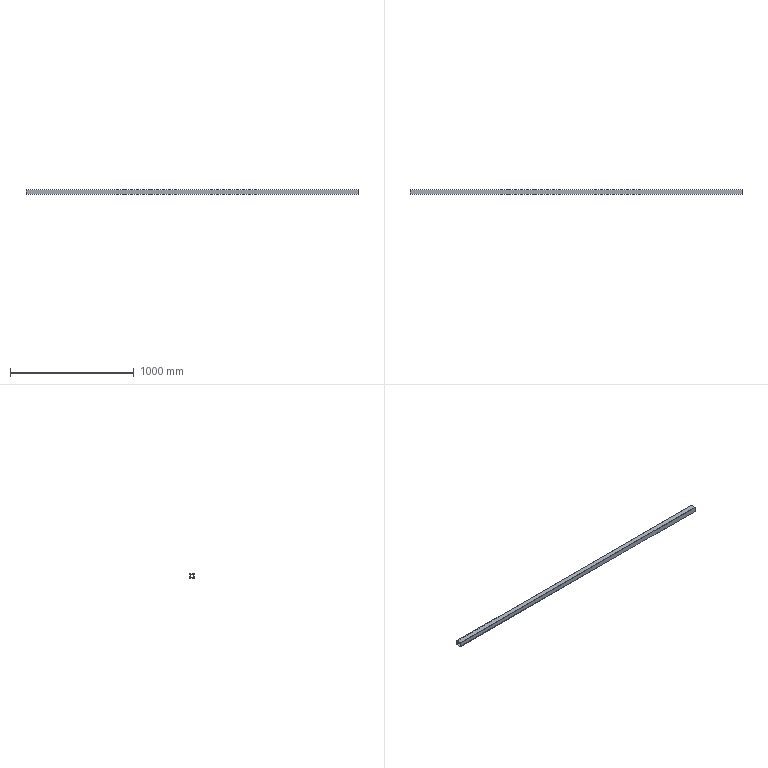Part | NX | features solid 2 | 1 solid | 10 faces | box 2680 x 40 x 40 mm | volume 1543680 mm3 | plane 10
STEP:
#1=CARTESIAN_POINT('',(1140.,-370.,-45.));
#2=VERTEX_POINT('',#1);
#3=CARTESIAN_POINT('',(1140.,-370.,-85.));
#4=VERTEX_POINT('',#3);
#5=CARTESIAN_POINT('',(1140.,-370.,-70.));
#6=DIRECTION('',(0.,0.,-1.));
#7=VECTOR('',#6,1000.);
#8=LINE('',#5,#7);
#9=EDGE_CURVE('',#2,#4,#8,.T.);
#10=ORIENTED_EDGE('',*,*,#9,.F.);
#11=CARTESIAN_POINT('',(-1540.,-370.,-45.));
#12=VERTEX_POINT('',#11);
#13=CARTESIAN_POINT('',(204.393,-370.,-45.));
#14=DIRECTION('',(1.,0.,0.));
#15=VECTOR('',#14,1000.);
#16=LINE('',#13,#15);
#17=EDGE_CURVE('',#12,#2,#16,.T.);
#18=ORIENTED_EDGE('',*,*,#17,.F.);
#19=CARTESIAN_POINT('',(-1540.,-370.,-85.));
#20=VERTEX_POINT('',#19);
#21=CARTESIAN_POINT('',(-1540.,-370.,-70.));
#22=DIRECTION('',(0.,0.,-1.));
#23=VECTOR('',#22,1000.);
#24=LINE('',#21,#23);
#25=EDGE_CURVE('',#12,#20,#24,.T.);
#26=ORIENTED_EDGE('',*,*,#25,.T.);
#27=CARTESIAN_POINT('',(119.393,-370.,-85.));
#28=DIRECTION('',(1.,0.,0.));
#29=VECTOR('',#28,1000.);
#30=LINE('',#27,#29);
#31=EDGE_CURVE('',#20,#4,#30,.T.);
#32=ORIENTED_EDGE('',*,*,#31,.T.);
#33=EDGE_LOOP('',(#10,#18,#26,#32));
#34=FACE_BOUND('',#33,.T.);
#35=CARTESIAN_POINT('',(119.393,-370.,-70.));
#36=DIRECTION('',(0.,1.,0.));
#37=DIRECTION('',(0.,0.,1.));
#38=AXIS2_PLACEMENT_3D('',#35,#36,#37);
#39=PLANE('',#38);
#40=ADVANCED_FACE('',(#34),#39,.F.);
#41=CARTESIAN_POINT('',(1140.,-330.,-85.));
#42=VERTEX_POINT('',#41);
#43=CARTESIAN_POINT('',(1140.,-950.,-85.));
#44=DIRECTION('',(0.,1.,0.));
#45=VECTOR('',#44,1000.);
#46=LINE('',#43,#45);
#47=EDGE_CURVE('',#4,#42,#46,.T.);
#48=ORIENTED_EDGE('',*,*,#47,.F.);
#49=ORIENTED_EDGE('',*,*,#31,.F.);
#50=CARTESIAN_POINT('',(-1540.,-330.,-85.));
#51=VERTEX_POINT('',#50);
#52=CARTESIAN_POINT('',(-1540.,-950.,-85.));
#53=DIRECTION('',(0.,1.,0.));
#54=VECTOR('',#53,1000.);
#55=LINE('',#52,#54);
#56=EDGE_CURVE('',#20,#51,#55,.T.);
#57=ORIENTED_EDGE('',*,*,#56,.T.);
#58=CARTESIAN_POINT('',(204.393,-330.,-85.));
#59=DIRECTION('',(1.,0.,0.));
#60=VECTOR('',#59,1000.);
#61=LINE('',#58,#60);
#62=EDGE_CURVE('',#51,#42,#61,.T.);
#63=ORIENTED_EDGE('',*,*,#62,.T.);
#64=EDGE_LOOP('',(#48,#49,#57,#63));
#65=FACE_BOUND('',#64,.T.);
#66=CARTESIAN_POINT('',(204.393,-950.,-85.));
#67=DIRECTION('',(0.,0.,1.));
#68=DIRECTION('',(0.,-1.,0.));
#69=AXIS2_PLACEMENT_3D('',#66,#67,#68);
#70=PLANE('',#69);
#71=ADVANCED_FACE('',(#65),#70,.F.);
#72=CARTESIAN_POINT('',(1140.,-330.,-45.));
#73=VERTEX_POINT('',#72);
#74=CARTESIAN_POINT('',(1140.,-990.,-45.));
#75=DIRECTION('',(0.,-1.,0.));
#76=VECTOR('',#75,1000.);
#77=LINE('',#74,#76);
#78=EDGE_CURVE('',#73,#2,#77,.T.);
#79=ORIENTED_EDGE('',*,*,#78,.F.);
#80=CARTESIAN_POINT('',(-1540.,-330.,-45.));
#81=VERTEX_POINT('',#80);
#82=CARTESIAN_POINT('',(204.393,-330.,-45.));
#83=DIRECTION('',(-1.,0.,0.));
#84=VECTOR('',#83,1000.);
#85=LINE('',#82,#84);
#86=EDGE_CURVE('',#73,#81,#85,.T.);
#87=ORIENTED_EDGE('',*,*,#86,.T.);
#88=CARTESIAN_POINT('',(-1540.,-990.,-45.));
#89=DIRECTION('',(0.,-1.,0.));
#90=VECTOR('',#89,1000.);
#91=LINE('',#88,#90);
#92=EDGE_CURVE('',#81,#12,#91,.T.);
#93=ORIENTED_EDGE('',*,*,#92,.T.);
#94=ORIENTED_EDGE('',*,*,#17,.T.);
#95=EDGE_LOOP('',(#79,#87,#93,#94));
#96=FACE_BOUND('',#95,.T.);
#97=CARTESIAN_POINT('',(204.393,-990.,-45.));
#98=DIRECTION('',(0.,0.,-1.));
#99=DIRECTION('',(0.,1.,0.));
#100=AXIS2_PLACEMENT_3D('',#97,#98,#99);
#101=PLANE('',#100);
#102=ADVANCED_FACE('',(#96),#101,.F.);
#103=CARTESIAN_POINT('',(1140.,-330.,-40.));
#104=DIRECTION('',(0.,0.,1.));
#105=VECTOR('',#104,1000.);
#106=LINE('',#103,#105);
#107=EDGE_CURVE('',#42,#73,#106,.T.);
#108=ORIENTED_EDGE('',*,*,#107,.F.);
#109=ORIENTED_EDGE('',*,*,#62,.F.);
#110=CARTESIAN_POINT('',(-1540.,-330.,-40.));
#111=DIRECTION('',(0.,0.,1.));
#112=VECTOR('',#111,1000.);
#113=LINE('',#110,#112);
#114=EDGE_CURVE('',#51,#81,#113,.T.);
#115=ORIENTED_EDGE('',*,*,#114,.T.);
#116=ORIENTED_EDGE('',*,*,#86,.F.);
#117=EDGE_LOOP('',(#108,#109,#115,#116));
#118=FACE_BOUND('',#117,.T.);
#119=CARTESIAN_POINT('',(119.393,-330.,-40.));
#120=DIRECTION('',(0.,-1.,0.));
#121=DIRECTION('',(0.,0.,-1.));
#122=AXIS2_PLACEMENT_3D('',#119,#120,#121);
#123=PLANE('',#122);
#124=ADVANCED_FACE('',(#118),#123,.F.);
#125=CARTESIAN_POINT('',(-1540.,-366.,-49.));
#126=VERTEX_POINT('',#125);
#127=CARTESIAN_POINT('',(1140.,-366.,-49.));
#128=VERTEX_POINT('',#127);
#129=CARTESIAN_POINT('',(204.393,-366.,-49.));
#130=DIRECTION('',(1.,0.,0.));
#131=VECTOR('',#130,1000.);
#132=LINE('',#129,#131);
#133=EDGE_CURVE('',#126,#128,#132,.T.);
#134=ORIENTED_EDGE('',*,*,#133,.T.);
#135=CARTESIAN_POINT('',(1140.,-366.,-81.));
#136=VERTEX_POINT('',#135);
#137=CARTESIAN_POINT('',(1140.,-366.,-70.));
#138=DIRECTION('',(0.,0.,-1.));
#139=VECTOR('',#138,1000.);
#140=LINE('',#137,#139);
#141=EDGE_CURVE('',#128,#136,#140,.T.);
#142=ORIENTED_EDGE('',*,*,#141,.T.);
#143=CARTESIAN_POINT('',(-1540.,-366.,-81.));
#144=VERTEX_POINT('',#143);
#145=CARTESIAN_POINT('',(119.393,-366.,-81.));
#146=DIRECTION('',(1.,0.,0.));
#147=VECTOR('',#146,1000.);
#148=LINE('',#145,#147);
#149=EDGE_CURVE('',#144,#136,#148,.T.);
#150=ORIENTED_EDGE('',*,*,#149,.F.);
#151=CARTESIAN_POINT('',(-1540.,-366.,-70.));
#152=DIRECTION('',(0.,0.,-1.));
#153=VECTOR('',#152,1000.);
#154=LINE('',#151,#153);
#155=EDGE_CURVE('',#126,#144,#154,.T.);
#156=ORIENTED_EDGE('',*,*,#155,.F.);
#157=EDGE_LOOP('',(#134,#142,#150,#156));
#158=FACE_BOUND('',#157,.T.);
#159=CARTESIAN_POINT('',(119.393,-366.,-70.));
#160=DIRECTION('',(0.,1.,0.));
#161=DIRECTION('',(0.,0.,1.));
#162=AXIS2_PLACEMENT_3D('',#159,#160,#161);
#163=PLANE('',#162);
#164=ADVANCED_FACE('',(#158),#163,.T.);
#165=ORIENTED_EDGE('',*,*,#149,.T.);
#166=CARTESIAN_POINT('',(1140.,-334.,-81.));
#167=VERTEX_POINT('',#166);
#168=CARTESIAN_POINT('',(1140.,-950.,-81.));
#169=DIRECTION('',(0.,1.,0.));
#170=VECTOR('',#169,1000.);
#171=LINE('',#168,#170);
#172=EDGE_CURVE('',#136,#167,#171,.T.);
#173=ORIENTED_EDGE('',*,*,#172,.T.);
#174=CARTESIAN_POINT('',(-1540.,-334.,-81.));
#175=VERTEX_POINT('',#174);
#176=CARTESIAN_POINT('',(204.393,-334.,-81.));
#177=DIRECTION('',(1.,0.,0.));
#178=VECTOR('',#177,1000.);
#179=LINE('',#176,#178);
#180=EDGE_CURVE('',#175,#167,#179,.T.);
#181=ORIENTED_EDGE('',*,*,#180,.F.);
#182=CARTESIAN_POINT('',(-1540.,-950.,-81.));
#183=DIRECTION('',(0.,1.,0.));
#184=VECTOR('',#183,1000.);
#185=LINE('',#182,#184);
#186=EDGE_CURVE('',#144,#175,#185,.T.);
#187=ORIENTED_EDGE('',*,*,#186,.F.);
#188=EDGE_LOOP('',(#165,#173,#181,#187));
#189=FACE_BOUND('',#188,.T.);
#190=CARTESIAN_POINT('',(204.393,-950.,-81.));
#191=DIRECTION('',(0.,0.,1.));
#192=DIRECTION('',(0.,-1.,0.));
#193=AXIS2_PLACEMENT_3D('',#190,#191,#192);
#194=PLANE('',#193);
#195=ADVANCED_FACE('',(#189),#194,.T.);
#196=CARTESIAN_POINT('',(1140.,-334.,-49.));
#197=VERTEX_POINT('',#196);
#198=CARTESIAN_POINT('',(-1540.,-334.,-49.));
#199=VERTEX_POINT('',#198);
#200=CARTESIAN_POINT('',(204.393,-334.,-49.));
#201=DIRECTION('',(-1.,0.,0.));
#202=VECTOR('',#201,1000.);
#203=LINE('',#200,#202);
#204=EDGE_CURVE('',#197,#199,#203,.T.);
#205=ORIENTED_EDGE('',*,*,#204,.F.);
#206=CARTESIAN_POINT('',(1140.,-990.,-49.));
#207=DIRECTION('',(0.,-1.,0.));
#208=VECTOR('',#207,1000.);
#209=LINE('',#206,#208);
#210=EDGE_CURVE('',#197,#128,#209,.T.);
#211=ORIENTED_EDGE('',*,*,#210,.T.);
#212=ORIENTED_EDGE('',*,*,#133,.F.);
#213=CARTESIAN_POINT('',(-1540.,-990.,-49.));
#214=DIRECTION('',(0.,-1.,0.));
#215=VECTOR('',#214,1000.);
#216=LINE('',#213,#215);
#217=EDGE_CURVE('',#199,#126,#216,.T.);
#218=ORIENTED_EDGE('',*,*,#217,.F.);
#219=EDGE_LOOP('',(#205,#211,#212,#218));
#220=FACE_BOUND('',#219,.T.);
#221=CARTESIAN_POINT('',(204.393,-990.,-49.));
#222=DIRECTION('',(0.,0.,-1.));
#223=DIRECTION('',(0.,1.,0.));
#224=AXIS2_PLACEMENT_3D('',#221,#222,#223);
#225=PLANE('',#224);
#226=ADVANCED_FACE('',(#220),#225,.T.);
#227=ORIENTED_EDGE('',*,*,#180,.T.);
#228=CARTESIAN_POINT('',(1140.,-334.,-40.));
#229=DIRECTION('',(0.,0.,1.));
#230=VECTOR('',#229,1000.);
#231=LINE('',#228,#230);
#232=EDGE_CURVE('',#167,#197,#231,.T.);
#233=ORIENTED_EDGE('',*,*,#232,.T.);
#234=ORIENTED_EDGE('',*,*,#204,.T.);
#235=CARTESIAN_POINT('',(-1540.,-334.,-40.));
#236=DIRECTION('',(0.,0.,1.));
#237=VECTOR('',#236,1000.);
#238=LINE('',#235,#237);
#239=EDGE_CURVE('',#175,#199,#238,.T.);
#240=ORIENTED_EDGE('',*,*,#239,.F.);
#241=EDGE_LOOP('',(#227,#233,#234,#240));
#242=FACE_BOUND('',#241,.T.);
#243=CARTESIAN_POINT('',(119.393,-334.,-40.));
#244=DIRECTION('',(0.,-1.,0.));
#245=DIRECTION('',(0.,0.,-1.));
#246=AXIS2_PLACEMENT_3D('',#243,#244,#245);
#247=PLANE('',#246);
#248=ADVANCED_FACE('',(#242),#247,.T.);
#249=ORIENTED_EDGE('',*,*,#217,.T.);
#250=ORIENTED_EDGE('',*,*,#155,.T.);
#251=ORIENTED_EDGE('',*,*,#186,.T.);
#252=ORIENTED_EDGE('',*,*,#239,.T.);
#253=EDGE_LOOP('',(#249,#250,#251,#252));
#254=FACE_BOUND('',#253,.T.);
#255=ORIENTED_EDGE('',*,*,#25,.F.);
#256=ORIENTED_EDGE('',*,*,#92,.F.);
#257=ORIENTED_EDGE('',*,*,#114,.F.);
#258=ORIENTED_EDGE('',*,*,#56,.F.);
#259=EDGE_LOOP('',(#255,#256,#257,#258));
#260=FACE_BOUND('',#259,.T.);
#261=CARTESIAN_POINT('',(-1540.,180.,-39.5));
#262=DIRECTION('',(1.,0.,0.));
#263=DIRECTION('',(0.,-1.,0.));
#264=AXIS2_PLACEMENT_3D('',#261,#262,#263);
#265=PLANE('',#264);
#266=ADVANCED_FACE('',(#254,#260),#265,.F.);
#267=ORIENTED_EDGE('',*,*,#141,.F.);
#268=ORIENTED_EDGE('',*,*,#210,.F.);
#269=ORIENTED_EDGE('',*,*,#232,.F.);
#270=ORIENTED_EDGE('',*,*,#172,.F.);
#271=EDGE_LOOP('',(#267,#268,#269,#270));
#272=FACE_BOUND('',#271,.T.);
#273=ORIENTED_EDGE('',*,*,#78,.T.);
#274=ORIENTED_EDGE('',*,*,#9,.T.);
#275=ORIENTED_EDGE('',*,*,#47,.T.);
#276=ORIENTED_EDGE('',*,*,#107,.T.);
#277=EDGE_LOOP('',(#273,#274,#275,#276));
#278=FACE_BOUND('',#277,.T.);
#279=CARTESIAN_POINT('',(1140.,-397.5,-9.5));
#280=DIRECTION('',(1.,0.,0.));
#281=DIRECTION('',(0.,0.,-1.));
#282=AXIS2_PLACEMENT_3D('',#279,#280,#281);
#283=PLANE('',#282);
#284=ADVANCED_FACE('',(#272,#278),#283,.T.);
#285=CLOSED_SHELL('',(#40,#71,#102,#124,#164,#195,#226,#248,#266,#284));
#286=MANIFOLD_SOLID_BREP('',#285);
#287=(LENGTH_UNIT()NAMED_UNIT(*)SI_UNIT(.MILLI.,.METRE.));
#288=UNCERTAINTY_MEASURE_WITH_UNIT(LENGTH_MEASURE(0.00001),#287,'','');
#289=(NAMED_UNIT(*)PLANE_ANGLE_UNIT()SI_UNIT($,.RADIAN.));
#290=(NAMED_UNIT(*)SI_UNIT($,.STERADIAN.)SOLID_ANGLE_UNIT());
#291=(GEOMETRIC_REPRESENTATION_CONTEXT(3)GLOBAL_UNCERTAINTY_ASSIGNED_CONTEXT((#288))GLOBAL_UNIT_ASSIGNED_CONTEXT((#287,#289,#290))REPRESENTATION_CONTEXT('',''));
#292=ADVANCED_BREP_SHAPE_REPRESENTATION('',(#286),#291);